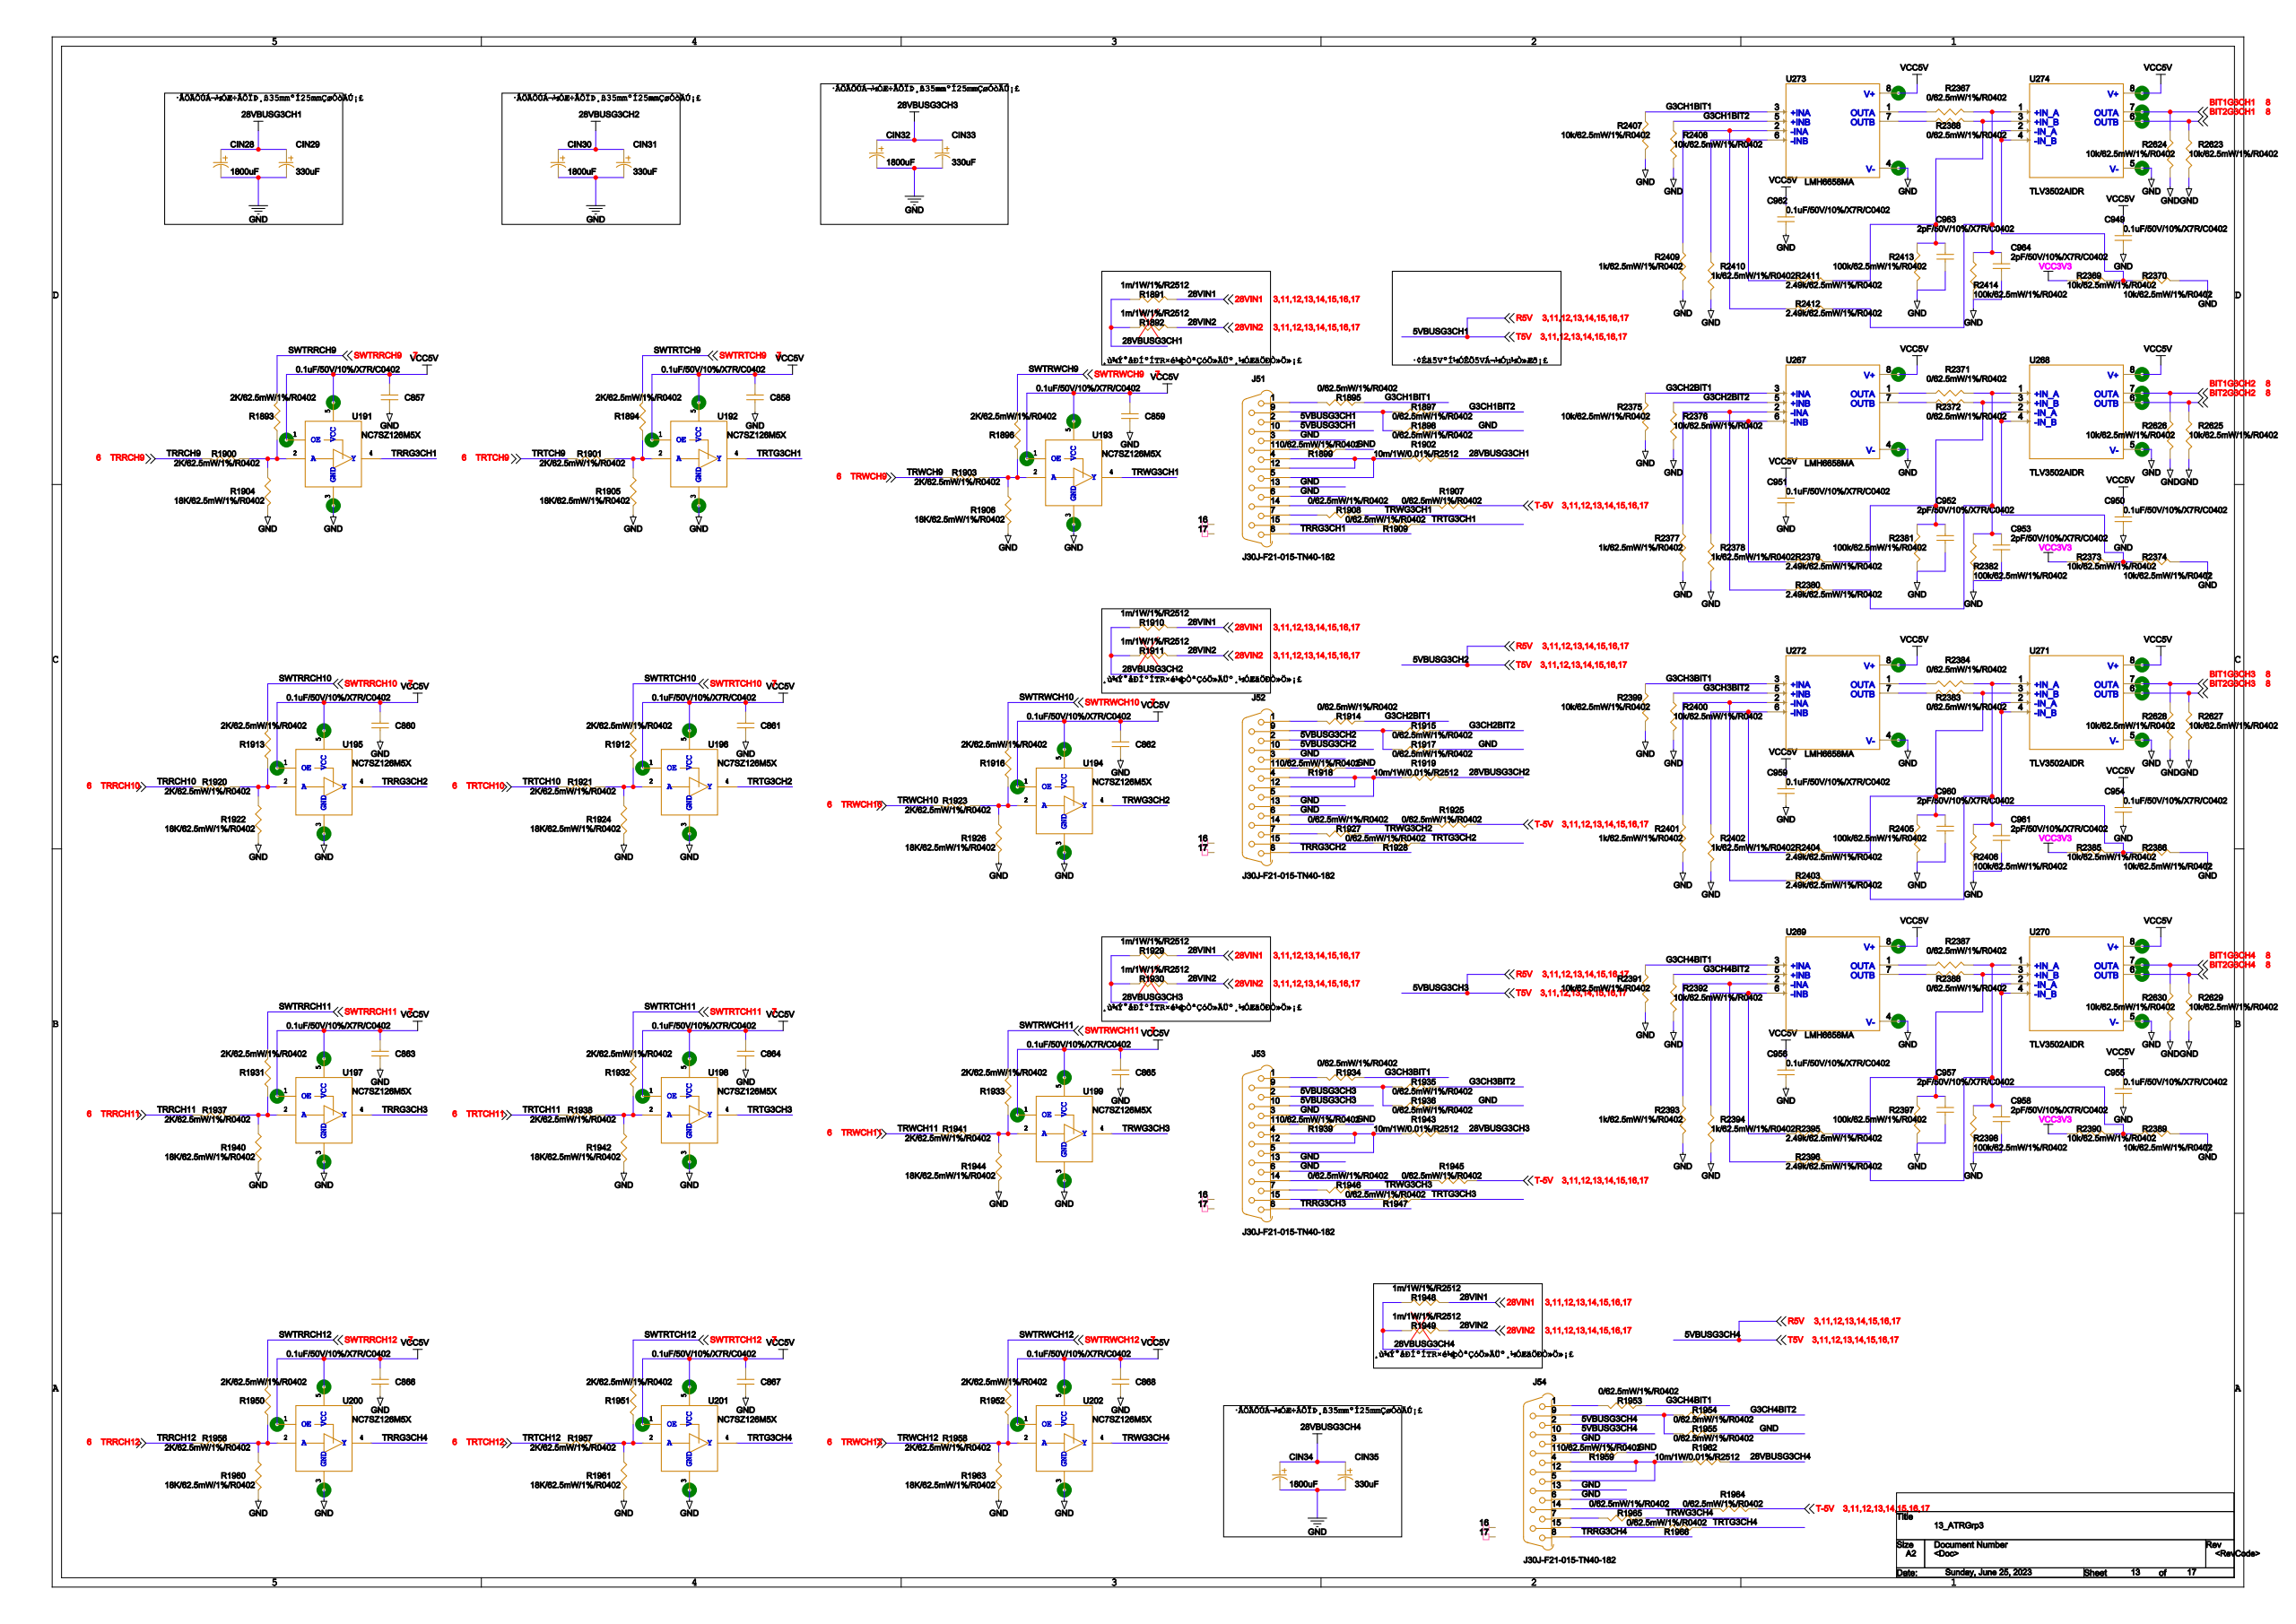Circuit board | Cadence Allegro | 1997 parts | 1536 nets | one sheet of the schematic
Parts on this sheet (reference | value | footprint):
C857 | 0.1uF/50V/10%/X7R/C0402 | 0402
C858 | 0.1uF/50V/10%/X7R/C0402 | 0402
C859 | 0.1uF/50V/10%/X7R/C0402 | 0402
C860 | 0.1uF/50V/10%/X7R/C0402 | 0402
C861 | 0.1uF/50V/10%/X7R/C0402 | 0402
C862 | 0.1uF/50V/10%/X7R/C0402 | 0402
C863 | 0.1uF/50V/10%/X7R/C0402 | 0402
C864 | 0.1uF/50V/10%/X7R/C0402 | 0402
C865 | 0.1uF/50V/10%/X7R/C0402 | 0402
C866 | 0.1uF/50V/10%/X7R/C0402 | 0402
C867 | 0.1uF/50V/10%/X7R/C0402 | 0402
C868 | 0.1uF/50V/10%/X7R/C0402 | 0402
C949 | 0.1uF/50V/10%/X7R/C0402 | 0402
C950 | 0.1uF/50V/10%/X7R/C0402 | 0402
C952 | 2pF/50V/10%/X7R/C0402 | 0402
C953 | 2pF/50V/10%/X7R/C0402 | 0402
C954 | 0.1uF/50V/10%/X7R/C0402 | 0402
C955 | 0.1uF/50V/10%/X7R/C0402 | 0402
C957 | 2pF/50V/10%/X7R/C0402 | 0402
C958 | 2pF/50V/10%/X7R/C0402 | 0402
C960 | 2pF/50V/10%/X7R/C0402 | 0402
C961 | 2pF/50V/10%/X7R/C0402 | 0402
C963 | 2pF/50V/10%/X7R/C0402 | 0402
C964 | 2pF/50V/10%/X7R/C0402 | 0402
CIN28 | ECF1HM182M27OTPO | AP-SMD_BD18-L27-W6_6-LS7_21
CIN29 | ECF1JM331G20OTPO | AP-SMD_BD10-L20-W6_6-LS7_21
CIN30 | ECF1HM182M27OTPO | AP-SMD_BD18-L27-W6_6-LS7_21
CIN31 | ECF1JM331G20OTPO | AP-SMD_BD10-L20-W6_6-LS7_21
CIN32 | ECF1HM182M27OTPO | AP-SMD_BD18-L27-W6_6-LS7_21
CIN33 | ECF1JM331G20OTPO | AP-SMD_BD10-L20-W6_6-LS7_21
CIN34 | ECF1HM182M27OTPO | AP-SMD_BD18-L27-W6_6-LS7_21
CIN35 | ECF1JM331G20OTPO | AP-SMD_BD10-L20-W6_6-LS7_21
J51 | J30J-F21-015-TN40-182 | J30J-F21-015-TN40-182
J52 | J30J-F21-015-TN40-182 | J30J-F21-015-TN40-182
J53 | J30J-F21-015-TN40-182 | J30J-F21-015-TN40-182
J54 | J30J-F21-015-TN40-182 | J30J-F21-015-TN40-182
R1891 | 1m/1W/1%/R2512 | 2512
R1892 | 1m/1W/1%/R2512 | 2512
R1893 | 2K/62.5mW/1%/R0402 | 0402
R1894 | 2K/62.5mW/1%/R0402 | 0402
R1895 | 0/62.5mW/1%/R0402 | 0402
R1896 | 2K/62.5mW/1%/R0402 | 0402
R1897 | 0/62.5mW/1%/R0402 | 0402
R1898 | 0/62.5mW/1%/R0402 | 0402
R1899 | 0/62.5mW/1%/R0402 | 0402
R1900 | 2K/62.5mW/1%/R0402 | 0402
R1901 | 2K/62.5mW/1%/R0402 | 0402
R1902 | 10m/1W/0.01%/R2512 | 2512
R1903 | 2K/62.5mW/1%/R0402 | 0402
R1904 | 18K/62.5mW/1%/R0402 | 0402
R1905 | 18K/62.5mW/1%/R0402 | 0402
R1906 | 18K/62.5mW/1%/R0402 | 0402
R1907 | 0/62.5mW/1%/R0402 | 0402
R1908 | 0/62.5mW/1%/R0402 | 0402
R1909 | 0/62.5mW/1%/R0402 | 0402
R1910 | 1m/1W/1%/R2512 | 2512
R1911 | 1m/1W/1%/R2512 | 2512
R1912 | 2K/62.5mW/1%/R0402 | 0402
R1913 | 2K/62.5mW/1%/R0402 | 0402
R1914 | 0/62.5mW/1%/R0402 | 0402
R1915 | 0/62.5mW/1%/R0402 | 0402
R1916 | 2K/62.5mW/1%/R0402 | 0402
R1917 | 0/62.5mW/1%/R0402 | 0402
R1918 | 0/62.5mW/1%/R0402 | 0402
R1919 | 10m/1W/0.01%/R2512 | 2512
R1920 | 2K/62.5mW/1%/R0402 | 0402
R1921 | 2K/62.5mW/1%/R0402 | 0402
R1922 | 18K/62.5mW/1%/R0402 | 0402
R1923 | 2K/62.5mW/1%/R0402 | 0402
R1924 | 18K/62.5mW/1%/R0402 | 0402
R1925 | 0/62.5mW/1%/R0402 | 0402
R1926 | 18K/62.5mW/1%/R0402 | 0402
R1927 | 0/62.5mW/1%/R0402 | 0402
R1928 | 0/62.5mW/1%/R0402 | 0402
R1929 | 1m/1W/1%/R2512 | 2512
R1930 | 1m/1W/1%/R2512 | 2512
R1931 | 2K/62.5mW/1%/R0402 | 0402
R1932 | 2K/62.5mW/1%/R0402 | 0402
R1933 | 2K/62.5mW/1%/R0402 | 0402
R1934 | 0/62.5mW/1%/R0402 | 0402
R1935 | 0/62.5mW/1%/R0402 | 0402
R1936 | 0/62.5mW/1%/R0402 | 0402
R1937 | 2K/62.5mW/1%/R0402 | 0402
R1938 | 2K/62.5mW/1%/R0402 | 0402
R1939 | 0/62.5mW/1%/R0402 | 0402
R1940 | 18K/62.5mW/1%/R0402 | 0402
R1941 | 2K/62.5mW/1%/R0402 | 0402
R1942 | 18K/62.5mW/1%/R0402 | 0402
R1943 | 10m/1W/0.01%/R2512 | 2512
R1944 | 18K/62.5mW/1%/R0402 | 0402
R1945 | 0/62.5mW/1%/R0402 | 0402
R1946 | 0/62.5mW/1%/R0402 | 0402
R1947 | 0/62.5mW/1%/R0402 | 0402
R1948 | 1m/1W/1%/R2512 | 2512
R1949 | 1m/1W/1%/R2512 | 2512
R1950 | 2K/62.5mW/1%/R0402 | 0402
R1951 | 2K/62.5mW/1%/R0402 | 0402
R1952 | 2K/62.5mW/1%/R0402 | 0402
R1953 | 0/62.5mW/1%/R0402 | 0402
R1954 | 0/62.5mW/1%/R0402 | 0402
R1955 | 0/62.5mW/1%/R0402 | 0402
R1956 | 2K/62.5mW/1%/R0402 | 0402
R1957 | 2K/62.5mW/1%/R0402 | 0402
R1958 | 2K/62.5mW/1%/R0402 | 0402
R1959 | 0/62.5mW/1%/R0402 | 0402
R1960 | 18K/62.5mW/1%/R0402 | 0402
R1961 | 18K/62.5mW/1%/R0402 | 0402
R1962 | 10m/1W/0.01%/R2512 | 2512
R1963 | 18K/62.5mW/1%/R0402 | 0402
R1964 | 0/62.5mW/1%/R0402 | 0402
R1965 | 0/62.5mW/1%/R0402 | 0402
R1966 | 0/62.5mW/1%/R0402 | 0402
R2367 | 0/62.5mW/1%/R0402 | 0402
R2368 | 0/62.5mW/1%/R0402 | 0402
R2369 | 10k/62.5mW/1%/R0402 | 0402
R2370 | 10k/62.5mW/1%/R0402 | 0402
R2371 | 0/62.5mW/1%/R0402 | 0402
R2372 | 0/62.5mW/1%/R0402 | 0402
R2373 | 10k/62.5mW/1%/R0402 | 0402
R2374 | 10k/62.5mW/1%/R0402 | 0402
R2375 | 10k/62.5mW/1%/R0402 | 0402
R2376 | 10k/62.5mW/1%/R0402 | 0402
R2377 | 1K/62.5mW/1%/R0402 | 0402
R2378 | 1K/62.5mW/1%/R0402 | 0402
R2380 | 2.49k/62.5mW/1%/R0402 | 0402
R2381 | 100k/62.5mW/1%/R0402 | 0402
R2382 | 100k/62.5mW/1%/R0402 | 0402
R2383 | 0/62.5mW/1%/R0402 | 0402
R2384 | 0/62.5mW/1%/R0402 | 0402
R2385 | 10k/62.5mW/1%/R0402 | 0402
R2386 | 10k/62.5mW/1%/R0402 | 0402
R2387 | 0/62.5mW/1%/R0402 | 0402
R2388 | 0/62.5mW/1%/R0402 | 0402
R2389 | 10k/62.5mW/1%/R0402 | 0402
R2390 | 10k/62.5mW/1%/R0402 | 0402
R2391 | 10k/62.5mW/1%/R0402 | 0402
R2392 | 10k/62.5mW/1%/R0402 | 0402
R2393 | 1K/62.5mW/1%/R0402 | 0402
R2394 | 1K/62.5mW/1%/R0402 | 0402
R2396 | 2.49k/62.5mW/1%/R0402 | 0402
R2397 | 100k/62.5mW/1%/R0402 | 0402
R2398 | 100k/62.5mW/1%/R0402 | 0402
R2399 | 10k/62.5mW/1%/R0402 | 0402
R2400 | 10k/62.5mW/1%/R0402 | 0402
R2401 | 1K/62.5mW/1%/R0402 | 0402
R2402 | 1K/62.5mW/1%/R0402 | 0402
R2403 | 2.49k/62.5mW/1%/R0402 | 0402
R2404 | 2.49k/62.5mW/1%/R0402 | 0402
R2405 | 100k/62.5mW/1%/R0402 | 0402
R2406 | 100k/62.5mW/1%/R0402 | 0402
R2407 | 10k/62.5mW/1%/R0402 | 0402
R2408 | 10k/62.5mW/1%/R0402 | 0402
R2409 | 1K/62.5mW/1%/R0402 | 0402
R2410 | 1K/62.5mW/1%/R0402 | 0402
R2412 | 2.49k/62.5mW/1%/R0402 | 0402
R2413 | 100k/62.5mW/1%/R0402 | 0402
R2414 | 100k/62.5mW/1%/R0402 | 0402
R2623 | 10k/62.5mW/1%/R0402 | 0402
R2624 | 10k/62.5mW/1%/R0402 | 0402
R2625 | 10k/62.5mW/1%/R0402 | 0402
R2626 | 10k/62.5mW/1%/R0402 | 0402
R2627 | 10k/62.5mW/1%/R0402 | 0402
R2628 | 10k/62.5mW/1%/R0402 | 0402
R2629 | 10k/62.5mW/1%/R0402 | 0402
R2630 | 10k/62.5mW/1%/R0402 | 0402
U191 | NC7SZ126M5X | SOT-23-5
U192 | NC7SZ126M5X | SOT-23-5
U193 | NC7SZ126M5X | SOT-23-5
U194 | NC7SZ126M5X | SOT-23-5
U195 | NC7SZ126M5X | SOT-23-5
U196 | NC7SZ126M5X | SOT-23-5
U197 | NC7SZ126M5X | SOT-23-5
U198 | NC7SZ126M5X | SOT-23-5
U199 | NC7SZ126M5X | SOT-23-5
U200 | NC7SZ126M5X | SOT-23-5
U201 | NC7SZ126M5X | SOT-23-5
U202 | NC7SZ126M5X | SOT-23-5
U267 | LMH6658MA | SOIC127P599X175-8N
U269 | LMH6658MA | SOIC127P599X175-8N
U271 | TLV3502AIDR | SOIC127P599X175-8N
U273 | LMH6658MA | SOIC127P599X175-8N
Nets of these parts (net: part-pin ...):
3.3V: R2369-1 R2373-1 R2385-1 R2390-1
AGND: C857-2 C858-2 C859-2 C860-2 C861-2 C862-2 C863-2 C864-2 C865-2 C866-2 C867-2 C868-2 C949-2 C950-2 C952-2 C953-2 C954-2 C955-2 C957-2 C958-2 C960-2 C961-2 C963-2 C964-2 CIN28-2 CIN29-2 CIN30-2 CIN31-2 CIN32-2 CIN33-2 CIN34-2 CIN35-2 J51-3 J51-6 J51-13 J52-3 J52-6 J52-13 J53-3 J53-6 J53-13 J54-3 J54-6 J54-13 R1898-1 R1899-1 R1904-1 R1905-1 R1906-1 R1917-1 R1918-1 R1922-1 R1924-1 R1926-1 R1936-1 R1939-1 R1940-1 R1942-1 R1944-1 R1955-1 R1959-1 R1960-1 R1961-1 R1963-1 R2370-2 R2374-2 R2375-2 R2376-2 R2377-2 R2378-2 R2381-2 R2382-2 R2386-2 R2389-2 R2391-2 R2392-2 R2393-2 R2394-2 R2397-2 R2398-2 R2399-2 R2400-2 R2401-2 R2402-2 R2405-2 R2406-2 R2407-2 R2408-2 R2409-2 R2410-2 R2413-2 R2414-2 R2623-2 R2624-2 R2625-2 R2626-2 R2627-2 R2628-2 R2629-2 R2630-2 U191-3 U192-3 U193-3 U194-3 U195-3 U196-3 U197-3 U198-3 U199-3 U200-3 U201-3 U202-3 U267-4 U269-4 U271-5 U273-4
VCC5V: C857-1 C858-1 C859-1 C860-1 C861-1 C862-1 C863-1 C864-1 C865-1 C866-1 C867-1 C868-1 C949-1 C950-1 C954-1 C955-1 U191-1 U191-5 U192-1 U192-5 U193-1 U193-5 U194-1 U194-5 U195-1 U195-5 U196-1 U196-5 U197-1 U197-5 U198-1 U198-5 U199-1 U199-5 U200-1 U200-5 U201-1 U201-5 U202-1 U202-5 U267-8 U269-8 U271-8 U273-8
N24399384: R2378-1 U267-6
N24399394: C952-1 R2372-2 R2381-1
N24399372: R2377-1 R2380-1 U267-2
N24399392: C953-1 R2371-2 R2380-2 R2382-1
N24399938: R2394-1 U269-6
N24399948: C957-1 R2388-2 R2397-1
N24399926: R2393-1 R2396-1 U269-2
N24399946: C958-1 R2387-2 R2396-2 R2398-1
N24399750: R2401-1 R2403-1
N24399766: C961-1 R2384-2 R2403-2 R2406-1 U271-1
N24399754: R2402-1 R2404-1
N24399768: C960-1 R2383-2 R2404-2 R2405-1 U271-3
N24399204: R2410-1 U273-6
N24399214: C963-1 R2368-2 R2413-1
N24399200: R2409-1 R2412-1 U273-2
N24399212: C964-1 R2367-2 R2412-2 R2414-1
G3CH2BIT1: R1914-1 R2375-1 U267-3
G3CH2BIT2: R1915-1 R2376-1 U267-5
N24399388: R2371-1 U267-1
N24399390: R2372-1 U267-7
G3CH4BIT1: R1953-1 R2391-1 U269-3
G3CH4BIT2: R1954-1 R2392-1 U269-5
N24399942: R2387-1 U269-1
N24399944: R2388-1 U269-7
G3CH3BIT1: R1934-1 R2399-1
G3CH3BIT2: R1935-1 R2400-1
N24399762: R2384-1
N24399764: R2383-1
G3CH1BIT1: R1895-1 R2407-1 U273-3
G3CH1BIT2: R1897-1 R2408-1 U273-5
N24399208: R2367-1 U273-1
N24399210: R2368-1 U273-7
N24399446: R2373-2 R2374-1
BIT1G3CH2: R2626-1
BIT2G3CH2: R2625-1
N24400000: R2389-1 R2390-2
BIT1G3CH4: R2630-1
BIT2G3CH4: R2629-1
N24399820: R2385-2 R2386-1 U271-2 U271-4
BIT1G3CH3: R2628-1 U271-7
BIT2G3CH3: R2627-1 U271-6
N24399266: R2369-2 R2370-1
BIT1G3CH1: R2624-1
BIT2G3CH1: R2623-1
R5V: J51-2 J51-10 J52-2 J52-10 J53-2 J53-10 J54-2 J54-10
N23725346: J51-1 R1895-2
N23725359: J51-11 R1899-2
N23725361: J51-4 J51-5 J51-12 R1902-1
N23725373: J51-14 R1907-2
N23725377: J51-15 R1909-2
N23725375: J51-7 R1908-2
TRRG3CH1: J51-8 U191-4
N23725348: J51-9 R1897-2 R1898-2
N23725905: J52-1 R1914-2
N23725918: J52-11 R1918-2
N23725920: J52-4 J52-5 J52-12 R1919-1
N23725932: J52-14 R1925-2
N23725936: J52-15 R1928-2
N23725934: J52-7 R1927-2
TRRG3CH2: J52-8 U195-4
N23725907: J52-9 R1915-2 R1917-2
N23726532: J53-1 R1934-2
N23726545: J53-11 R1939-2
N23726547: J53-4 J53-5 J53-12 R1943-1
N23726559: J53-14 R1945-2
N23726563: J53-15 R1947-2
N23726561: J53-7 R1946-2
TRRG3CH3: J53-8 U197-4
N23726534: J53-9 R1935-2 R1936-2
N23727336: J54-1 R1953-2
N23727349: J54-11 R1959-2
N23727351: J54-4 J54-5 J54-12 R1962-1
N23727363: J54-14 R1964-2
N23727367: J54-15 R1966-2
N23727365: J54-7 R1965-2
TRRG3CH4: J54-8 U200-4
N23727338: J54-9 R1954-2 R1955-2
28VIN1: R1891-2 R1910-2 R1929-2 R1948-2
T-5V: R1907-1 R1925-1 R1945-1 R1964-1
28VIN2: R1892-2 R1911-2 R1930-2 R1949-2
28VBUSG3CH1: CIN28-1 CIN29-1 R1891-1 R1892-1 R1902-2
28VBUSG3CH2: CIN30-1 CIN31-1 R1910-1 R1911-1 R1919-2
28VBUSG3CH3: CIN32-1 CIN33-1 R1929-1 R1930-1 R1943-2
28VBUSG3CH4: CIN34-1 CIN35-1 R1948-1 R1949-1 R1962-2
SWTRRCH9: R1893-1
N24007480: R1893-2 R1900-2 R1904-2 U191-2
SWTRTCH9: R1894-1
N24006500: R1894-2 R1901-2 R1905-2 U192-2
SWTRWCH9: R1896-1
N24006988: R1896-2 R1903-2 R1906-2 U193-2
TRRCH9: R1900-1
TRTCH9: R1901-1
TRWCH9: R1903-1
SWTRTCH10: R1912-1
N24006618: R1912-2 R1921-2 R1924-2 U196-2
SWTRRCH10: R1913-1
N24007598: R1913-2 R1920-2 R1922-2 U195-2
SWTRWCH10: R1916-1
N24007110: R1916-2 R1923-2 R1926-2 U194-2
TRRCH10: R1920-1
TRTCH10: R1921-1
TRWCH10: R1923-1
SWTRRCH11: R1931-1
N24007724: R1931-2 R1937-2 R1940-2 U197-2
SWTRTCH11: R1932-1
N24006744: R1932-2 R1938-2 R1942-2 U198-2
SWTRWCH11: R1933-1
N24007232: R1933-2 R1941-2 R1944-2 U199-2
TRRCH11: R1937-1
TRTCH11: R1938-1
TRWCH11: R1941-1
SWTRRCH12: R1950-1
N24007842: R1950-2 R1956-2 R1960-2 U200-2
SWTRTCH12: R1951-1
N24006866: R1951-2 R1957-2 R1961-2 U201-2
SWTRWCH12: R1952-1
N24007354: R1952-2 R1958-2 R1963-2 U202-2
TRRCH12: R1956-1
TRTCH12: R1957-1
TRWCH12: R1958-1
TRTG3CH1: R1909-1 U192-4
TRWG3CH1: R1908-1 U193-4
TRWG3CH2: R1927-1 U194-4
TRTG3CH2: R1928-1 U196-4
TRTG3CH3: R1947-1 U198-4
TRWG3CH3: R1946-1 U199-4
TRTG3CH4: R1966-1 U201-4
TRWG3CH4: R1965-1 U202-4